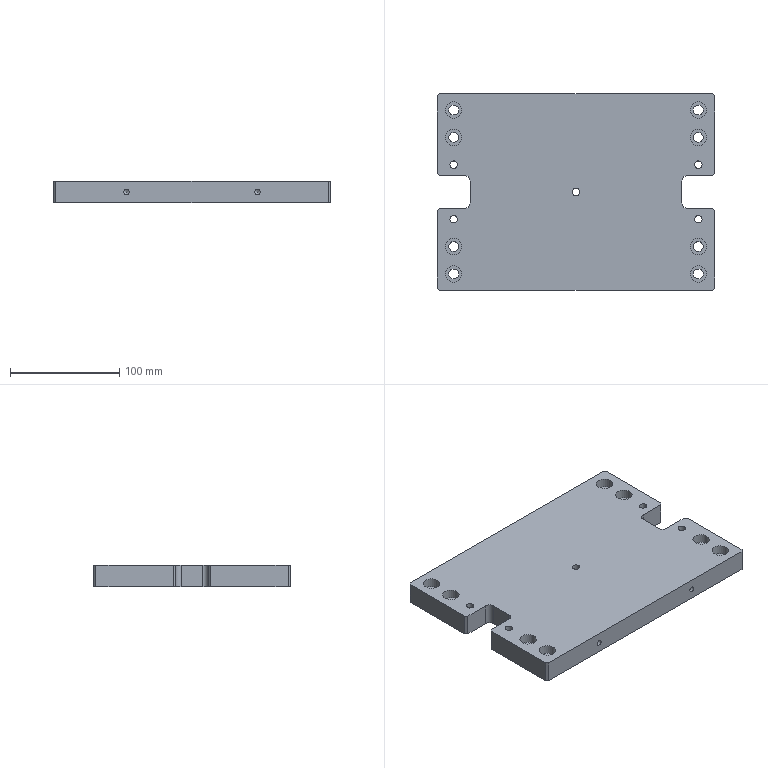CAM job | NX | 3-axis milling, drilling | part box 254 x 180 x 20 mm | stock box 254 x 180 x 20 mm
Tools:
number,name,description,diameter,corner_radius,flute_length,length,flutes
6,D6,平底铣刀-粗,6.0,0.0,25.0,75.0,2
9,D10,平底铣刀-粗,10.0,0.0,35.0,75.0,2
7,D6-J,平底铣刀-精,6.0,0.0,25.0,75.0,2
10,D10-J,平底铣刀-精,10.0,0.0,35.0,75.0,2
2,D6倒角刀,倒角刀,6.0,0.0,3.0,25.0,2
22,M8X1.25,丝锥,6.8,0.0,35.0,50.0,2
1,C6定点钻,倒角刀,6.0,0.0,3.0,3.0,2
17,ZT9,钻头,9.0,0.0,35.0,50.0,2
16,ZT6.9,Drilling Tool,6.9,0.0,35.0,50.0,2
Operations:
program,operation,operation_type,tool,method,geometry_group,spindle_rpm,surface_speed,feed_per_tooth,feed_cut,feed_plunge,cut_length_mm,path_length_mm,cut_time_min,machine_time_min
B,选线往复层切开粗-中_COPY_2,PlanarMilling,D10,分层开粗-切深K-步距G,W-B,3000.0,94.245,0.3333,2000.0,100.0,1832.902,2791.326,0.9165,1.012
B,铣倒角_2,PlanarMilling,D6倒角刀,METHOD,W-B,4000.0,75.398,0.0375,300.0,100.0,119.577,760.164,0.3986,0.4626
B,平面去毛刺6X45L_COPY_1,SurfaceContour,D6倒角刀,爬面_倒角-切深0-步距G,W-B,3500.0,65.972,0.1429,1000.0,100.0,1280.472,2265.924,1.28,1.379
B,平面铣精光侧面-中-直线_COPY_2,PlanarMilling,D10-J,侧刃精光-切深K-步距G,W-B,3000.0,94.245,0.1333,800.0,100.0,67.314,985.071,0.0841,0.1759
A,选线往复层切开粗-中_COPY,PlanarMilling,D10,分层开粗-切深K-步距G,W-A,3000.0,94.245,0.3333,2000.0,100.0,1832.902,2791.326,0.9165,1.012
A,选线往复层切开粗-中_COPY_1,PlanarMilling,D10,分层开粗-切深K-步距G,W-A,3000.0,94.245,0.3333,2000.0,100.0,19648.119,20122.459,9.824,9.871
A,打点-深0.8,Operation,C6定点钻,NONE,W-A,3000.0,56.0,0.01,60.0,90.0,23.4,688.572,0.39,0.4565
A,通孔-M8螺纹底孔,Operation,ZT6.9,NONE,W-A,600.0,12.818,0.1,120.0,90.0,135.0,663.541,1.125,1.178
A,沉头孔-钻孔0段,Operation,ZT9,NONE,W-A,500.0,14.137,0.12,120.0,90.0,205.631,1002.354,1.714,1.793
A,底壁铣螺旋开粗-中_COPY,VolumeBased25DMillingOperation,D6,分层开粗-切深K-步距G,W-A,4000.0,75.396,0.25,2000.0,100.0,9895.698,11064.622,4.948,5.065
A,铣倒角_1,PlanarMilling,D6倒角刀,METHOD,W-A,4000.0,75.398,0.0625,500.0,100.0,117.385,756.972,0.2348,0.2987
A,平面去毛刺6X45L_COPY,SurfaceContour,D6倒角刀,爬面_倒角-切深0-步距G,W-A,3500.0,65.972,0.1429,1000.0,100.0,1736.9,3435.226,1.737,1.907
A,通孔-攻牙M8,Operation,M8X1.25,METHOD,W-A,300.0,6.409,0.0021,1.25,90.0,125.0,643.541,100.0,100.052
A,底壁铣螺旋精光-中_COPY,VolumeBased25DMillingOperation,D6-J,螺旋精光-切深K-步距G,W-A,3500.0,65.972,0.1143,800.0,100.0,772.843,1931.874,0.9661,1.082
A,平面铣精光侧面-中-直线_COPY,PlanarMilling,D10-J,侧刃精光-切深K-步距G,W-A,3000.0,94.245,0.1333,800.0,100.0,67.314,985.071,0.0841,0.1759
A,平面铣精光侧面-中-直线_COPY_1,PlanarMilling,D10-J,侧刃精光-切深K-步距G,W-A,3000.0,94.245,0.1333,800.0,100.0,561.065,1497.078,0.7013,0.7949